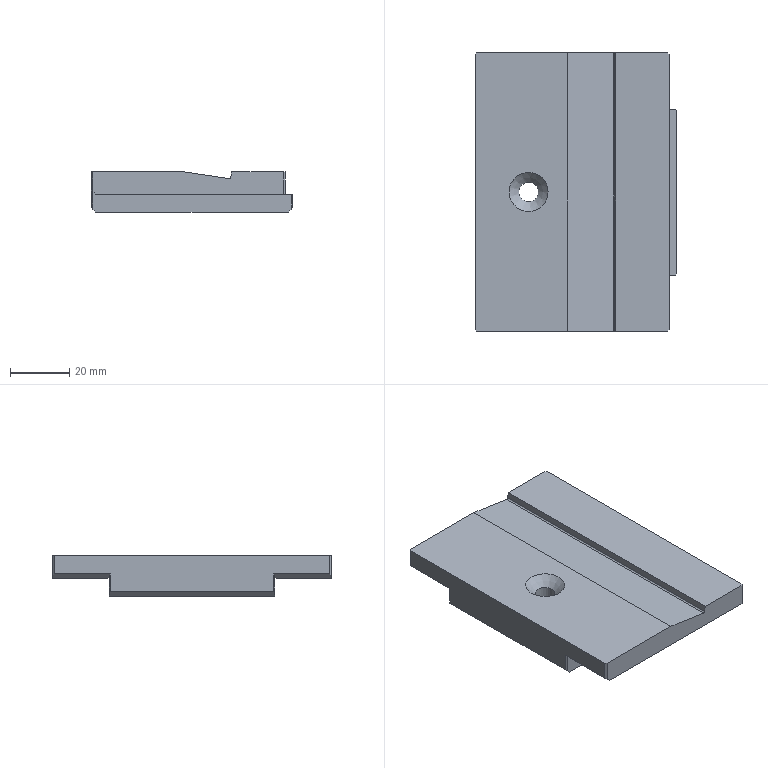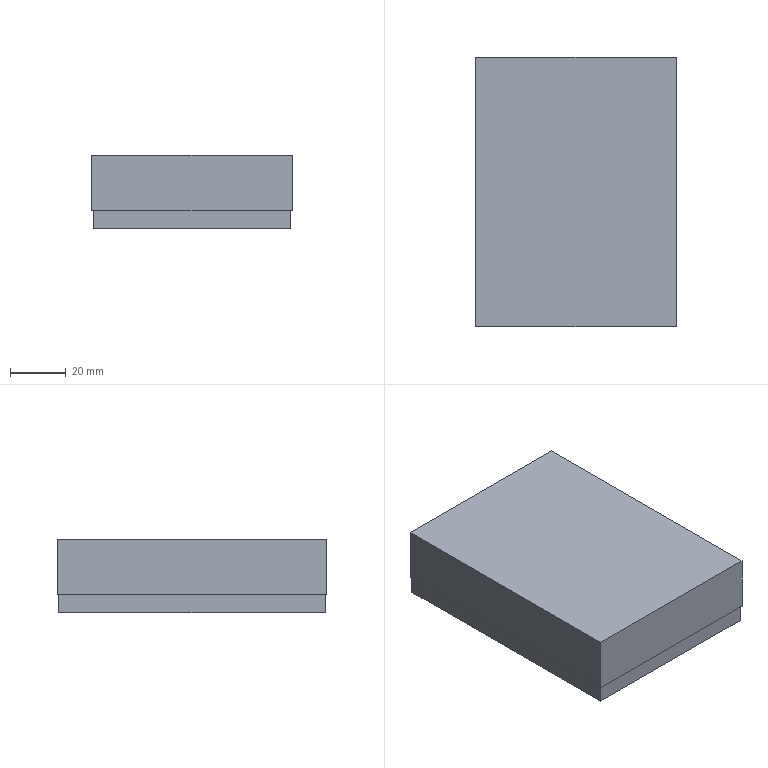CAM job | NX | 3+2 milling, drilling | part box 68 x 94 x 13.65 mm | stock box 72 x 97 x 26.35 mm
Tools:
number,name,description,diameter,corner_radius,flute_length,length,flutes
2,D12开粗,D12,12.0,0.0,30.0,75.0,2
3,D12精光,D12,12.0,0.0,30.0,75.0,2
7,D4R0.5,圆鼻铣刀,4.0,0.5,12.0,50.0,2
4,D4倒角刀,DJ4-32,4.0,0.0,2.0,50.0,2
1,D50面刀,Milling Tool-5 Parameters,50.0,0.0,50.0,75.0,2
8,D6.6钻头,Drilling Tool,6.6,0.0,35.0,50.0,2
Operations:
program,operation,operation_type,tool,method,geometry_group,spindle_rpm,surface_speed,feed_per_tooth,feed_cut,feed_plunge,cut_length_mm,path_length_mm,cut_time_min,machine_time_min
XX-CNC1,一刀光面,VolumeBased25DMillingOperation,D50面刀,METHOD,MCS_1,3500.0,1187.0,0.1,800.0,100.0,326.0,595.416,0.4075,0.4344
XX-CNC1,ADAPTIVE_MILLING,CavityMilling,D12开粗,METHOD,W1,6500.0,245.0,0.1923,2500.0,100.0,2551.234,3338.986,0.8525,0.9312
XX-CNC1,PLANAR_MILL,PlanarMilling,D12精光,METHOD,W1,5500.0,207.0,0.0727,800.0,100.0,524.128,772.727,0.6552,0.68
XX-CNC1,PLANAR_MILL_COPY,PlanarMilling,D12精光,METHOD,W1,5500.0,207.0,0.0727,800.0,100.0,253.678,545.71,0.3171,0.3463
XX-CNC1,PLANAR_MILL_COPY_COPY,PlanarMilling,D12精光,METHOD,W1,5500.0,207.0,0.0727,800.0,100.0,156.0,405.985,0.195,0.22
XX-CNC1,DRILLING,Operation,D4倒角刀,METHOD,W1,3000.0,37.0,0.0333,200.0,0.0,4.5,69.0,0.0225,0.0289
XX-CNC1,PLANAR_MILL_1,PlanarMilling,D4倒角刀,METHOD,W1,3500.0,100.0,0.1178,1000.0,100.0,334.685,393.685,0.3347,0.3406
XX-CNC1,DRILLING_COPY,Operation,D6.6钻头,METHOD,W1,3000.0,37.0,0.0333,200.0,0.0,21.0,102.0,0.105,0.1131
XX-CNC1,CURVE_DRIVE,SurfaceContour,D4R0.5,METHOD,W1,6500.0,81.0,0.0769,1000.0,100.0,729.452,785.193,0.7295,0.735
XX-CNC1,CURVE_DRIVE_COPY,SurfaceContour,D4R0.5,METHOD,W1,6500.0,81.0,0.2308,3000.0,100.0,11960.27,12014.789,3.987,3.992
XX-CNC1,CURVE_DRIVE_COPY_COPY,SurfaceContour,D4R0.5,METHOD,W1,6500.0,81.0,0.2308,3000.0,100.0,1327.376,1382.005,0.4425,0.4479
XX-CNC2,FLOOR_FACING,VolumeBased25DMillingOperation,D12开粗,METHOD,MCS_2,6500.0,245.0,0.0769,1000.0,100.0,231.403,285.203,0.2314,0.2368
XX-CNC2,PLANAR_MILL_2,PlanarMilling,D4R0.5,METHOD,MCS_2,6500.0,100.0,0.1178,1000.0,100.0,539.997,1207.795,0.54,0.6068
XX-CNC2,PLANAR_MILL_2_COPY,PlanarMilling,D4R0.5,METHOD,MCS_2,6500.0,100.0,0.1178,800.0,100.0,108.0,162.0,0.135,0.1404
XX-CNC2,FLOOR_FACING_COPY,VolumeBased25DMillingOperation,D4R0.5,METHOD,MCS_2,6500.0,245.0,0.0769,1000.0,100.0,809.7,863.7,0.8097,0.8151
XX-CNC3,ADAPTIVE_MILLING_1,CavityMilling,D12开粗,METHOD,W3,6500.0,100.0,0.1178,3000.0,100.0,13600.318,14333.311,4.487,4.56
XX-CNC3,FLOOR_FACING_1,VolumeBased25DMillingOperation,D12精光,METHOD,W3,5500.0,207.0,0.0727,800.0,100.0,1113.997,1468.542,1.393,1.428
XX-CNC3,FLOOR_FACING_1_COPY,VolumeBased25DMillingOperation,D12精光,METHOD,W3,5500.0,207.0,0.0727,800.0,100.0,168.912,372.912,0.2111,0.2315
XX-CNC3,PLANAR_MILL_3,PlanarMilling,D4倒角刀,METHOD,W3,4500.0,56.0,0.1111,1000.0,100.0,152.0,328.6,0.152,0.1697
XX-CNC3,PLANAR_MILL_3_COPY_1,PlanarMilling,D4倒角刀,METHOD,W3,4500.0,56.0,0.0333,300.0,100.0,21.708,80.708,0.0724,0.0783
XX-CNC3,PLANAR_MILL_3_COPY,PlanarMilling,D4倒角刀,METHOD,W3,4500.0,56.0,0.1111,1000.0,100.0,272.0,707.201,0.272,0.3155
XX-CNC3,PLANAR_MILL_3_COPY_COPY,PlanarMilling,D4倒角刀,METHOD,W3,4500.0,56.0,0.1111,1000.0,100.0,177.21,380.21,0.1772,0.1975
XX-CNC3,等高爬角,ZLevelMilling,D4R0.5,METHOD,W3,6000.0,188.496,0.25,3000.0,90.0,1509.281,1731.983,0.5034,0.5256